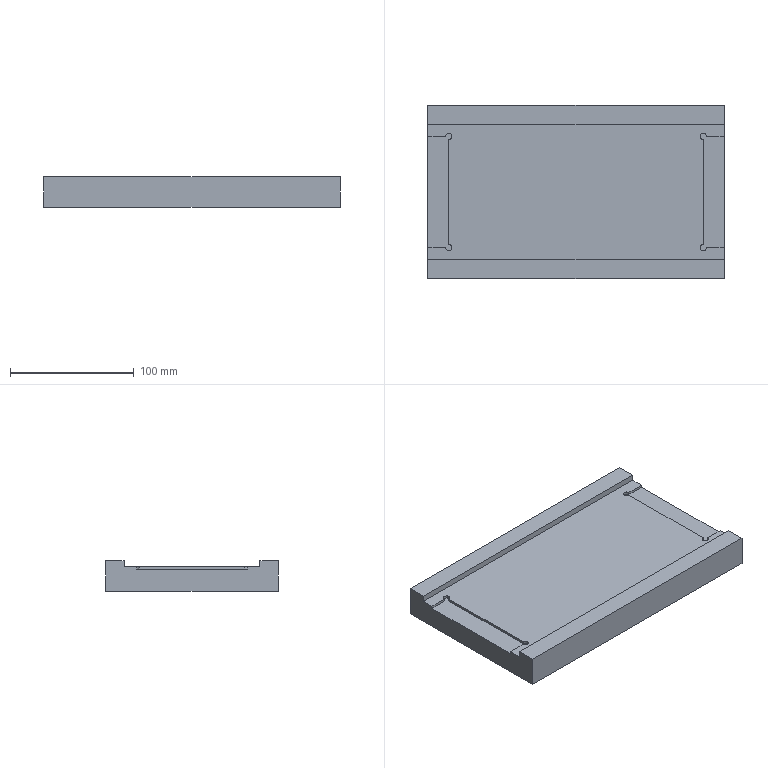Part | STEP file | 001-009-Riveting guide plate | 1 solid | 24 faces | box 240 x 140 x 25 mm | volume 701762 mm3 | plane 18 | cylinder 6 | commonest cylinder face diameters 5 x6